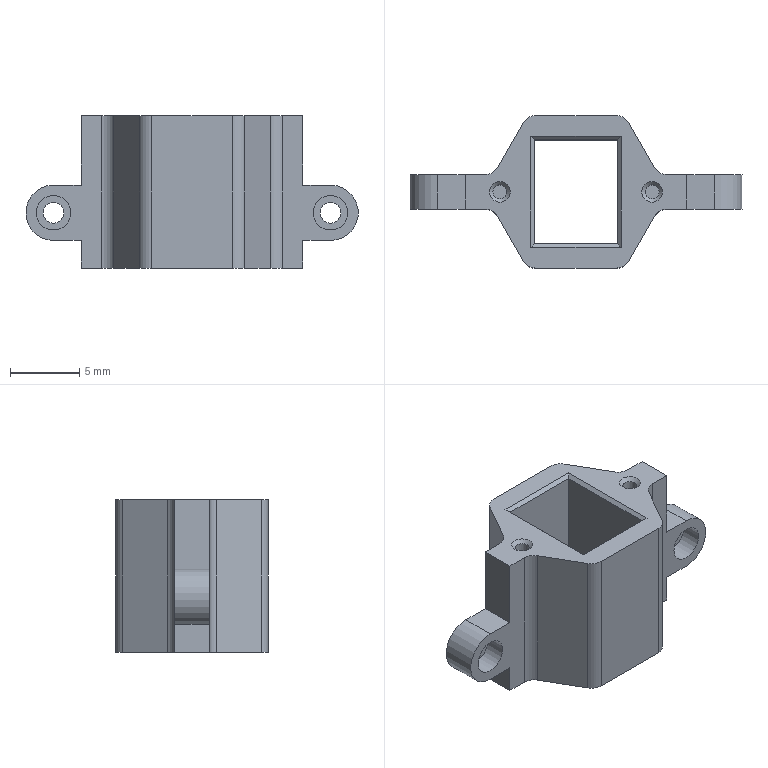Part | NX | features DATUM_CSYS 4, EXTRUDE 3, SKETCH 3, CBORE_HOLE 2, HOLE PACKAGE 2, BLEND 1, CHAMFER 1, SCALE 1 | 1 solid | 50 faces | box 24 x 11 x 11 mm | volume 869.205 mm3 | plane 32 | cylinder 16 | cone 2 | commonest cylinder face diameters 2 x8 1 x2 1.5 x2 2.5 x2 4 x2
STEP:
#1=CARTESIAN_POINT('',(-8.,-1.25,6.));
#2=VERTEX_POINT('',#1);
#3=CARTESIAN_POINT('',(-8.,1.25,6.));
#4=VERTEX_POINT('',#3);
#5=CARTESIAN_POINT('',(-8.,-1.25,6.));
#6=DIRECTION('',(0.,1.,0.));
#7=VECTOR('',#6,1000.);
#8=LINE('',#5,#7);
#9=EDGE_CURVE('',#2,#4,#8,.T.);
#10=ORIENTED_EDGE('',*,*,#9,.F.);
#11=CARTESIAN_POINT('',(-8.,-1.25,11.));
#12=VERTEX_POINT('',#11);
#13=CARTESIAN_POINT('',(-8.,-1.25,11.));
#14=DIRECTION('',(0.,0.,-1.));
#15=VECTOR('',#14,1000.);
#16=LINE('',#13,#15);
#17=EDGE_CURVE('',#12,#2,#16,.T.);
#18=ORIENTED_EDGE('',*,*,#17,.F.);
#19=CARTESIAN_POINT('',(-8.,1.25,11.));
#20=VERTEX_POINT('',#19);
#21=CARTESIAN_POINT('',(-8.,1.25,11.));
#22=DIRECTION('',(0.,-1.,0.));
#23=VECTOR('',#22,1000.);
#24=LINE('',#21,#23);
#25=EDGE_CURVE('',#20,#12,#24,.T.);
#26=ORIENTED_EDGE('',*,*,#25,.F.);
#27=CARTESIAN_POINT('',(-8.,1.25,11.));
#28=DIRECTION('',(0.,0.,-1.));
#29=VECTOR('',#28,1000.);
#30=LINE('',#27,#29);
#31=EDGE_CURVE('',#20,#4,#30,.T.);
#32=ORIENTED_EDGE('',*,*,#31,.T.);
#33=EDGE_LOOP('',(#10,#18,#26,#32));
#34=FACE_BOUND('',#33,.T.);
#35=CARTESIAN_POINT('',(-8.,1.25,11.));
#36=DIRECTION('',(1.,0.,0.));
#37=DIRECTION('',(0.,0.,-1.));
#38=AXIS2_PLACEMENT_3D('',#35,#36,#37);
#39=PLANE('',#38);
#40=ADVANCED_FACE('',(#34),#39,.F.);
#41=CARTESIAN_POINT('',(8.,-1.25,2.));
#42=VERTEX_POINT('',#41);
#43=CARTESIAN_POINT('',(8.,1.25,2.));
#44=VERTEX_POINT('',#43);
#45=CARTESIAN_POINT('',(8.,-1.25,2.));
#46=DIRECTION('',(0.,1.,0.));
#47=VECTOR('',#46,1000.);
#48=LINE('',#45,#47);
#49=EDGE_CURVE('',#42,#44,#48,.T.);
#50=ORIENTED_EDGE('',*,*,#49,.F.);
#51=CARTESIAN_POINT('',(8.,-1.25,0.));
#52=VERTEX_POINT('',#51);
#53=CARTESIAN_POINT('',(8.,-1.25,11.));
#54=DIRECTION('',(0.,0.,-1.));
#55=VECTOR('',#54,1000.);
#56=LINE('',#53,#55);
#57=EDGE_CURVE('',#42,#52,#56,.T.);
#58=ORIENTED_EDGE('',*,*,#57,.T.);
#59=CARTESIAN_POINT('',(8.,1.25,0.));
#60=VERTEX_POINT('',#59);
#61=CARTESIAN_POINT('',(8.,-1.25,0.));
#62=DIRECTION('',(0.,1.,0.));
#63=VECTOR('',#62,1000.);
#64=LINE('',#61,#63);
#65=EDGE_CURVE('',#52,#60,#64,.T.);
#66=ORIENTED_EDGE('',*,*,#65,.T.);
#67=CARTESIAN_POINT('',(8.,1.25,11.));
#68=DIRECTION('',(0.,0.,-1.));
#69=VECTOR('',#68,1000.);
#70=LINE('',#67,#69);
#71=EDGE_CURVE('',#44,#60,#70,.T.);
#72=ORIENTED_EDGE('',*,*,#71,.F.);
#73=EDGE_LOOP('',(#50,#58,#66,#72));
#74=FACE_BOUND('',#73,.T.);
#75=CARTESIAN_POINT('',(8.,-1.25,11.));
#76=DIRECTION('',(-1.,0.,0.));
#77=DIRECTION('',(0.,0.,1.));
#78=AXIS2_PLACEMENT_3D('',#75,#76,#77);
#79=PLANE('',#78);
#80=ADVANCED_FACE('',(#74),#79,.F.);
#81=CARTESIAN_POINT('',(-3.,3.75,10.75));
#82=VERTEX_POINT('',#81);
#83=CARTESIAN_POINT('',(-3.,3.75,0.));
#84=VERTEX_POINT('',#83);
#85=CARTESIAN_POINT('',(-3.,3.75,11.));
#86=DIRECTION('',(0.,0.,-1.));
#87=VECTOR('',#86,1000.);
#88=LINE('',#85,#87);
#89=EDGE_CURVE('',#82,#84,#88,.T.);
#90=ORIENTED_EDGE('',*,*,#89,.F.);
#91=CARTESIAN_POINT('',(-3.,-3.75,10.75));
#92=VERTEX_POINT('',#91);
#93=CARTESIAN_POINT('',(-3.,-3.75,10.75));
#94=DIRECTION('',(0.,-1.,0.));
#95=VECTOR('',#94,1000.);
#96=LINE('',#93,#95);
#97=EDGE_CURVE('',#82,#92,#96,.T.);
#98=ORIENTED_EDGE('',*,*,#97,.T.);
#99=CARTESIAN_POINT('',(-3.,-3.75,0.));
#100=VERTEX_POINT('',#99);
#101=CARTESIAN_POINT('',(-3.,-3.75,11.));
#102=DIRECTION('',(0.,0.,-1.));
#103=VECTOR('',#102,1000.);
#104=LINE('',#101,#103);
#105=EDGE_CURVE('',#92,#100,#104,.T.);
#106=ORIENTED_EDGE('',*,*,#105,.T.);
#107=CARTESIAN_POINT('',(-3.,-3.75,0.));
#108=DIRECTION('',(0.,1.,0.));
#109=VECTOR('',#108,1000.);
#110=LINE('',#107,#109);
#111=EDGE_CURVE('',#100,#84,#110,.T.);
#112=ORIENTED_EDGE('',*,*,#111,.T.);
#113=EDGE_LOOP('',(#90,#98,#106,#112));
#114=FACE_BOUND('',#113,.T.);
#115=CARTESIAN_POINT('',(-3.,-3.75,11.));
#116=DIRECTION('',(-1.,0.,0.));
#117=DIRECTION('',(0.,0.,1.));
#118=AXIS2_PLACEMENT_3D('',#115,#116,#117);
#119=PLANE('',#118);
#120=ADVANCED_FACE('',(#114),#119,.F.);
#121=CARTESIAN_POINT('',(3.,3.75,10.75));
#122=VERTEX_POINT('',#121);
#123=CARTESIAN_POINT('',(3.,3.75,0.));
#124=VERTEX_POINT('',#123);
#125=CARTESIAN_POINT('',(3.,3.75,11.));
#126=DIRECTION('',(0.,0.,-1.));
#127=VECTOR('',#126,1000.);
#128=LINE('',#125,#127);
#129=EDGE_CURVE('',#122,#124,#128,.T.);
#130=ORIENTED_EDGE('',*,*,#129,.F.);
#131=CARTESIAN_POINT('',(-3.,3.75,10.75));
#132=DIRECTION('',(-1.,0.,0.));
#133=VECTOR('',#132,1000.);
#134=LINE('',#131,#133);
#135=EDGE_CURVE('',#122,#82,#134,.T.);
#136=ORIENTED_EDGE('',*,*,#135,.T.);
#137=ORIENTED_EDGE('',*,*,#89,.T.);
#138=CARTESIAN_POINT('',(-3.,3.75,0.));
#139=DIRECTION('',(1.,0.,0.));
#140=VECTOR('',#139,1000.);
#141=LINE('',#138,#140);
#142=EDGE_CURVE('',#84,#124,#141,.T.);
#143=ORIENTED_EDGE('',*,*,#142,.T.);
#144=EDGE_LOOP('',(#130,#136,#137,#143));
#145=FACE_BOUND('',#144,.T.);
#146=CARTESIAN_POINT('',(-3.,3.75,11.));
#147=DIRECTION('',(0.,1.,0.));
#148=DIRECTION('',(0.,0.,1.));
#149=AXIS2_PLACEMENT_3D('',#146,#147,#148);
#150=PLANE('',#149);
#151=ADVANCED_FACE('',(#145),#150,.F.);
#152=CARTESIAN_POINT('',(3.,-3.75,10.75));
#153=VERTEX_POINT('',#152);
#154=CARTESIAN_POINT('',(3.,-3.75,0.));
#155=VERTEX_POINT('',#154);
#156=CARTESIAN_POINT('',(3.,-3.75,11.));
#157=DIRECTION('',(0.,0.,-1.));
#158=VECTOR('',#157,1000.);
#159=LINE('',#156,#158);
#160=EDGE_CURVE('',#153,#155,#159,.T.);
#161=ORIENTED_EDGE('',*,*,#160,.F.);
#162=CARTESIAN_POINT('',(3.,3.75,10.75));
#163=DIRECTION('',(0.,1.,0.));
#164=VECTOR('',#163,1000.);
#165=LINE('',#162,#164);
#166=EDGE_CURVE('',#153,#122,#165,.T.);
#167=ORIENTED_EDGE('',*,*,#166,.T.);
#168=ORIENTED_EDGE('',*,*,#129,.T.);
#169=CARTESIAN_POINT('',(3.,3.75,0.));
#170=DIRECTION('',(0.,-1.,0.));
#171=VECTOR('',#170,1000.);
#172=LINE('',#169,#171);
#173=EDGE_CURVE('',#124,#155,#172,.T.);
#174=ORIENTED_EDGE('',*,*,#173,.T.);
#175=EDGE_LOOP('',(#161,#167,#168,#174));
#176=FACE_BOUND('',#175,.T.);
#177=CARTESIAN_POINT('',(3.,3.75,11.));
#178=DIRECTION('',(1.,0.,0.));
#179=DIRECTION('',(0.,0.,-1.));
#180=AXIS2_PLACEMENT_3D('',#177,#178,#179);
#181=PLANE('',#180);
#182=ADVANCED_FACE('',(#176),#181,.F.);
#183=CARTESIAN_POINT('',(-8.,-1.25,2.));
#184=VERTEX_POINT('',#183);
#185=CARTESIAN_POINT('',(-8.,-1.25,0.));
#186=VERTEX_POINT('',#185);
#187=CARTESIAN_POINT('',(-8.,-1.25,11.));
#188=DIRECTION('',(0.,0.,-1.));
#189=VECTOR('',#188,1000.);
#190=LINE('',#187,#189);
#191=EDGE_CURVE('',#184,#186,#190,.T.);
#192=ORIENTED_EDGE('',*,*,#191,.F.);
#193=CARTESIAN_POINT('',(-8.,1.25,2.));
#194=VERTEX_POINT('',#193);
#195=CARTESIAN_POINT('',(-8.,-1.25,2.));
#196=DIRECTION('',(0.,1.,0.));
#197=VECTOR('',#196,1000.);
#198=LINE('',#195,#197);
#199=EDGE_CURVE('',#184,#194,#198,.T.);
#200=ORIENTED_EDGE('',*,*,#199,.T.);
#201=CARTESIAN_POINT('',(-8.,1.25,0.));
#202=VERTEX_POINT('',#201);
#203=CARTESIAN_POINT('',(-8.,1.25,11.));
#204=DIRECTION('',(0.,0.,-1.));
#205=VECTOR('',#204,1000.);
#206=LINE('',#203,#205);
#207=EDGE_CURVE('',#194,#202,#206,.T.);
#208=ORIENTED_EDGE('',*,*,#207,.T.);
#209=CARTESIAN_POINT('',(-8.,1.25,0.));
#210=DIRECTION('',(0.,-1.,0.));
#211=VECTOR('',#210,1000.);
#212=LINE('',#209,#211);
#213=EDGE_CURVE('',#202,#186,#212,.T.);
#214=ORIENTED_EDGE('',*,*,#213,.T.);
#215=EDGE_LOOP('',(#192,#200,#208,#214));
#216=FACE_BOUND('',#215,.T.);
#217=CARTESIAN_POINT('',(-8.,1.25,11.));
#218=DIRECTION('',(1.,0.,0.));
#219=DIRECTION('',(0.,0.,-1.));
#220=AXIS2_PLACEMENT_3D('',#217,#218,#219);
#221=PLANE('',#220);
#222=ADVANCED_FACE('',(#216),#221,.F.);
#223=CARTESIAN_POINT('',(-11.25,-1.25,4.));
#224=VERTEX_POINT('',#223);
#225=CARTESIAN_POINT('',(-10.,-1.25,4.));
#226=DIRECTION('',(0.,1.,0.));
#227=DIRECTION('',(-1.,0.,0.));
#228=AXIS2_PLACEMENT_3D('',#225,#226,#227);
#229=CIRCLE('',#228,1.25);
#230=EDGE_CURVE('',#224,#224,#229,.T.);
#231=ORIENTED_EDGE('',*,*,#230,.T.);
#232=EDGE_LOOP('',(#231));
#233=FACE_BOUND('',#232,.T.);
#234=CARTESIAN_POINT('',(-6.531,-1.25,0.));
#235=VERTEX_POINT('',#234);
#236=CARTESIAN_POINT('',(-8.,-1.25,0.));
#237=DIRECTION('',(1.,0.,0.));
#238=VECTOR('',#237,1000.);
#239=LINE('',#236,#238);
#240=EDGE_CURVE('',#186,#235,#239,.T.);
#241=ORIENTED_EDGE('',*,*,#240,.T.);
#242=CARTESIAN_POINT('',(-6.531,-1.25,11.));
#243=VERTEX_POINT('',#242);
#244=CARTESIAN_POINT('',(-6.531,-1.25,11.));
#245=DIRECTION('',(0.,0.,-1.));
#246=VECTOR('',#245,1000.);
#247=LINE('',#244,#246);
#248=EDGE_CURVE('',#235,#243,#247,.F.);
#249=ORIENTED_EDGE('',*,*,#248,.T.);
#250=CARTESIAN_POINT('',(-8.,-1.25,11.));
#251=DIRECTION('',(1.,0.,0.));
#252=VECTOR('',#251,1000.);
#253=LINE('',#250,#252);
#254=EDGE_CURVE('',#12,#243,#253,.T.);
#255=ORIENTED_EDGE('',*,*,#254,.F.);
#256=ORIENTED_EDGE('',*,*,#17,.T.);
#257=CARTESIAN_POINT('',(-10.,-1.25,6.));
#258=VERTEX_POINT('',#257);
#259=CARTESIAN_POINT('',(-8.,-1.25,6.));
#260=DIRECTION('',(-1.,0.,0.));
#261=VECTOR('',#260,1000.);
#262=LINE('',#259,#261);
#263=EDGE_CURVE('',#2,#258,#262,.T.);
#264=ORIENTED_EDGE('',*,*,#263,.T.);
#265=CARTESIAN_POINT('',(-10.,-1.25,2.));
#266=VERTEX_POINT('',#265);
#267=CARTESIAN_POINT('',(-10.,-1.25,4.));
#268=DIRECTION('',(0.,-1.,0.));
#269=DIRECTION('',(-1.,0.,0.));
#270=AXIS2_PLACEMENT_3D('',#267,#268,#269);
#271=CIRCLE('',#270,2.);
#272=EDGE_CURVE('',#258,#266,#271,.T.);
#273=ORIENTED_EDGE('',*,*,#272,.T.);
#274=CARTESIAN_POINT('',(-10.,-1.25,2.));
#275=DIRECTION('',(1.,0.,0.));
#276=VECTOR('',#275,1000.);
#277=LINE('',#274,#276);
#278=EDGE_CURVE('',#266,#184,#277,.T.);
#279=ORIENTED_EDGE('',*,*,#278,.T.);
#280=ORIENTED_EDGE('',*,*,#191,.T.);
#281=EDGE_LOOP('',(#241,#249,#255,#256,#264,#273,#279,#280));
#282=FACE_BOUND('',#281,.T.);
#283=CARTESIAN_POINT('',(-8.,-1.25,11.));
#284=DIRECTION('',(0.,1.,0.));
#285=DIRECTION('',(-1.,0.,0.));
#286=AXIS2_PLACEMENT_3D('',#283,#284,#285);
#287=PLANE('',#286);
#288=ADVANCED_FACE('',(#233,#282),#287,.F.);
#289=CARTESIAN_POINT('',(-5.665,-1.75,11.));
#290=VERTEX_POINT('',#289);
#291=CARTESIAN_POINT('',(-3.789,-5.,11.));
#292=VERTEX_POINT('',#291);
#293=CARTESIAN_POINT('',(-5.954,-1.25,11.));
#294=DIRECTION('',(0.5,-0.866,0.));
#295=VECTOR('',#294,1000.);
#296=LINE('',#293,#295);
#297=EDGE_CURVE('',#290,#292,#296,.T.);
#298=ORIENTED_EDGE('',*,*,#297,.F.);
#299=CARTESIAN_POINT('',(-5.665,-1.75,0.));
#300=VERTEX_POINT('',#299);
#301=CARTESIAN_POINT('',(-5.665,-1.75,0.));
#302=DIRECTION('',(0.,0.,-1.));
#303=VECTOR('',#302,1000.);
#304=LINE('',#301,#303);
#305=EDGE_CURVE('',#290,#300,#304,.T.);
#306=ORIENTED_EDGE('',*,*,#305,.T.);
#307=CARTESIAN_POINT('',(-3.789,-5.,0.));
#308=VERTEX_POINT('',#307);
#309=CARTESIAN_POINT('',(-5.954,-1.25,0.));
#310=DIRECTION('',(0.5,-0.866,0.));
#311=VECTOR('',#310,1000.);
#312=LINE('',#309,#311);
#313=EDGE_CURVE('',#300,#308,#312,.T.);
#314=ORIENTED_EDGE('',*,*,#313,.T.);
#315=CARTESIAN_POINT('',(-3.789,-5.,11.));
#316=DIRECTION('',(0.,0.,-1.));
#317=VECTOR('',#316,1000.);
#318=LINE('',#315,#317);
#319=EDGE_CURVE('',#308,#292,#318,.F.);
#320=ORIENTED_EDGE('',*,*,#319,.T.);
#321=EDGE_LOOP('',(#298,#306,#314,#320));
#322=FACE_BOUND('',#321,.T.);
#323=CARTESIAN_POINT('',(-5.954,-1.25,11.));
#324=DIRECTION('',(0.866,0.5,0.));
#325=DIRECTION('',(-0.5,0.866,0.));
#326=AXIS2_PLACEMENT_3D('',#323,#324,#325);
#327=PLANE('',#326);
#328=ADVANCED_FACE('',(#322),#327,.F.);
#329=CARTESIAN_POINT('',(-2.923,-5.5,0.));
#330=VERTEX_POINT('',#329);
#331=CARTESIAN_POINT('',(2.923,-5.5,0.));
#332=VERTEX_POINT('',#331);
#333=CARTESIAN_POINT('',(-3.5,-5.5,0.));
#334=DIRECTION('',(1.,0.,0.));
#335=VECTOR('',#334,1000.);
#336=LINE('',#333,#335);
#337=EDGE_CURVE('',#330,#332,#336,.T.);
#338=ORIENTED_EDGE('',*,*,#337,.T.);
#339=CARTESIAN_POINT('',(2.923,-5.5,11.));
#340=VERTEX_POINT('',#339);
#341=CARTESIAN_POINT('',(2.923,-5.5,11.));
#342=DIRECTION('',(0.,0.,-1.));
#343=VECTOR('',#342,1000.);
#344=LINE('',#341,#343);
#345=EDGE_CURVE('',#332,#340,#344,.F.);
#346=ORIENTED_EDGE('',*,*,#345,.T.);
#347=CARTESIAN_POINT('',(-2.923,-5.5,11.));
#348=VERTEX_POINT('',#347);
#349=CARTESIAN_POINT('',(-3.5,-5.5,11.));
#350=DIRECTION('',(1.,0.,0.));
#351=VECTOR('',#350,1000.);
#352=LINE('',#349,#351);
#353=EDGE_CURVE('',#348,#340,#352,.T.);
#354=ORIENTED_EDGE('',*,*,#353,.F.);
#355=CARTESIAN_POINT('',(-2.923,-5.5,11.));
#356=DIRECTION('',(0.,0.,-1.));
#357=VECTOR('',#356,1000.);
#358=LINE('',#355,#357);
#359=EDGE_CURVE('',#348,#330,#358,.T.);
#360=ORIENTED_EDGE('',*,*,#359,.T.);
#361=EDGE_LOOP('',(#338,#346,#354,#360));
#362=FACE_BOUND('',#361,.T.);
#363=CARTESIAN_POINT('',(-3.5,-5.5,11.));
#364=DIRECTION('',(0.,1.,0.));
#365=DIRECTION('',(0.,0.,1.));
#366=AXIS2_PLACEMENT_3D('',#363,#364,#365);
#367=PLANE('',#366);
#368=ADVANCED_FACE('',(#362),#367,.F.);
#369=CARTESIAN_POINT('',(3.789,-5.,0.));
#370=VERTEX_POINT('',#369);
#371=CARTESIAN_POINT('',(5.665,-1.75,0.));
#372=VERTEX_POINT('',#371);
#373=CARTESIAN_POINT('',(3.5,-5.5,0.));
#374=DIRECTION('',(0.5,0.866,0.));
#375=VECTOR('',#374,1000.);
#376=LINE('',#373,#375);
#377=EDGE_CURVE('',#370,#372,#376,.T.);
#378=ORIENTED_EDGE('',*,*,#377,.T.);
#379=CARTESIAN_POINT('',(5.665,-1.75,11.));
#380=VERTEX_POINT('',#379);
#381=CARTESIAN_POINT('',(5.665,-1.75,11.));
#382=DIRECTION('',(0.,0.,-1.));
#383=VECTOR('',#382,1000.);
#384=LINE('',#381,#383);
#385=EDGE_CURVE('',#372,#380,#384,.F.);
#386=ORIENTED_EDGE('',*,*,#385,.T.);
#387=CARTESIAN_POINT('',(3.789,-5.,11.));
#388=VERTEX_POINT('',#387);
#389=CARTESIAN_POINT('',(3.5,-5.5,11.));
#390=DIRECTION('',(0.5,0.866,0.));
#391=VECTOR('',#390,1000.);
#392=LINE('',#389,#391);
#393=EDGE_CURVE('',#388,#380,#392,.T.);
#394=ORIENTED_EDGE('',*,*,#393,.F.);
#395=CARTESIAN_POINT('',(3.789,-5.,11.));
#396=DIRECTION('',(0.,0.,-1.));
#397=VECTOR('',#396,1000.);
#398=LINE('',#395,#397);
#399=EDGE_CURVE('',#388,#370,#398,.T.);
#400=ORIENTED_EDGE('',*,*,#399,.T.);
#401=EDGE_LOOP('',(#378,#386,#394,#400));
#402=FACE_BOUND('',#401,.T.);
#403=CARTESIAN_POINT('',(3.5,-5.5,11.));
#404=DIRECTION('',(-0.866,0.5,0.));
#405=DIRECTION('',(-0.5,-0.866,0.));
#406=AXIS2_PLACEMENT_3D('',#403,#404,#405);
#407=PLANE('',#406);
#408=ADVANCED_FACE('',(#402),#407,.F.);
#409=CARTESIAN_POINT('',(8.75,-1.25,4.));
#410=VERTEX_POINT('',#409);
#411=CARTESIAN_POINT('',(10.,-1.25,4.));
#412=DIRECTION('',(0.,1.,0.));
#413=DIRECTION('',(-1.,0.,0.));
#414=AXIS2_PLACEMENT_3D('',#411,#412,#413);
#415=CIRCLE('',#414,1.25);
#416=EDGE_CURVE('',#410,#410,#415,.T.);
#417=ORIENTED_EDGE('',*,*,#416,.T.);
#418=EDGE_LOOP('',(#417));
#419=FACE_BOUND('',#418,.T.);
#420=CARTESIAN_POINT('',(6.531,-1.25,11.));
#421=VERTEX_POINT('',#420);
#422=CARTESIAN_POINT('',(8.,-1.25,11.));
#423=VERTEX_POINT('',#422);
#424=CARTESIAN_POINT('',(5.954,-1.25,11.));
#425=DIRECTION('',(1.,0.,0.));
#426=VECTOR('',#425,1000.);
#427=LINE('',#424,#426);
#428=EDGE_CURVE('',#421,#423,#427,.T.);
#429=ORIENTED_EDGE('',*,*,#428,.F.);
#430=CARTESIAN_POINT('',(6.531,-1.25,0.));
#431=VERTEX_POINT('',#430);
#432=CARTESIAN_POINT('',(6.531,-1.25,0.));
#433=DIRECTION('',(0.,0.,-1.));
#434=VECTOR('',#433,1000.);
#435=LINE('',#432,#434);
#436=EDGE_CURVE('',#421,#431,#435,.T.);
#437=ORIENTED_EDGE('',*,*,#436,.T.);
#438=CARTESIAN_POINT('',(5.954,-1.25,0.));
#439=DIRECTION('',(1.,0.,0.));
#440=VECTOR('',#439,1000.);
#441=LINE('',#438,#440);
#442=EDGE_CURVE('',#431,#52,#441,.T.);
#443=ORIENTED_EDGE('',*,*,#442,.T.);
#444=ORIENTED_EDGE('',*,*,#57,.F.);
#445=CARTESIAN_POINT('',(10.,-1.25,2.));
#446=VERTEX_POINT('',#445);
#447=CARTESIAN_POINT('',(10.,-1.25,2.));
#448=DIRECTION('',(-1.,0.,0.));
#449=VECTOR('',#448,1000.);
#450=LINE('',#447,#449);
#451=EDGE_CURVE('',#446,#42,#450,.T.);
#452=ORIENTED_EDGE('',*,*,#451,.F.);
#453=CARTESIAN_POINT('',(10.,-1.25,6.));
#454=VERTEX_POINT('',#453);
#455=CARTESIAN_POINT('',(10.,-1.25,4.));
#456=DIRECTION('',(0.,1.,0.));
#457=DIRECTION('',(1.,0.,0.));
#458=AXIS2_PLACEMENT_3D('',#455,#456,#457);
#459=CIRCLE('',#458,2.);
#460=EDGE_CURVE('',#454,#446,#459,.T.);
#461=ORIENTED_EDGE('',*,*,#460,.F.);
#462=CARTESIAN_POINT('',(8.,-1.25,6.));
#463=VERTEX_POINT('',#462);
#464=CARTESIAN_POINT('',(8.,-1.25,6.));
#465=DIRECTION('',(1.,0.,0.));
#466=VECTOR('',#465,1000.);
#467=LINE('',#464,#466);
#468=EDGE_CURVE('',#463,#454,#467,.T.);
#469=ORIENTED_EDGE('',*,*,#468,.F.);
#470=CARTESIAN_POINT('',(8.,-1.25,11.));
#471=DIRECTION('',(0.,0.,-1.));
#472=VECTOR('',#471,1000.);
#473=LINE('',#470,#472);
#474=EDGE_CURVE('',#423,#463,#473,.T.);
#475=ORIENTED_EDGE('',*,*,#474,.F.);
#476=EDGE_LOOP('',(#429,#437,#443,#444,#452,#461,#469,#475));
#477=FACE_BOUND('',#476,.T.);
#478=CARTESIAN_POINT('',(5.954,-1.25,11.));
#479=DIRECTION('',(0.,1.,0.));
#480=DIRECTION('',(-1.,0.,0.));
#481=AXIS2_PLACEMENT_3D('',#478,#479,#480);
#482=PLANE('',#481);
#483=ADVANCED_FACE('',(#419,#477),#482,.F.);
#484=ORIENTED_EDGE('',*,*,#474,.T.);
#485=CARTESIAN_POINT('',(8.,1.25,6.));
#486=VERTEX_POINT('',#485);
#487=CARTESIAN_POINT('',(8.,-1.25,6.));
#488=DIRECTION('',(0.,1.,0.));
#489=VECTOR('',#488,1000.);
#490=LINE('',#487,#489);
#491=EDGE_CURVE('',#463,#486,#490,.T.);
#492=ORIENTED_EDGE('',*,*,#491,.T.);
#493=CARTESIAN_POINT('',(8.,1.25,11.));
#494=VERTEX_POINT('',#493);
#495=CARTESIAN_POINT('',(8.,1.25,11.));
#496=DIRECTION('',(0.,0.,-1.));
#497=VECTOR('',#496,1000.);
#498=LINE('',#495,#497);
#499=EDGE_CURVE('',#494,#486,#498,.T.);
#500=ORIENTED_EDGE('',*,*,#499,.F.);
#501=CARTESIAN_POINT('',(8.,-1.25,11.));
#502=DIRECTION('',(0.,1.,0.));
#503=VECTOR('',#502,1000.);
#504=LINE('',#501,#503);
#505=EDGE_CURVE('',#423,#494,#504,.T.);
#506=ORIENTED_EDGE('',*,*,#505,.F.);
#507=EDGE_LOOP('',(#484,#492,#500,#506));
#508=FACE_BOUND('',#507,.T.);
#509=CARTESIAN_POINT('',(8.,-1.25,11.));
#510=DIRECTION('',(-1.,0.,0.));
#511=DIRECTION('',(0.,0.,1.));
#512=AXIS2_PLACEMENT_3D('',#509,#510,#511);
#513=PLANE('',#512);
#514=ADVANCED_FACE('',(#508),#513,.F.);
#515=CARTESIAN_POINT('',(10.75,1.25,4.));
#516=VERTEX_POINT('',#515);
#517=CARTESIAN_POINT('',(10.,1.25,4.));
#518=DIRECTION('',(0.,-1.,0.));
#519=DIRECTION('',(1.,0.,0.));
#520=AXIS2_PLACEMENT_3D('',#517,#518,#519);
#521=CIRCLE('',#520,0.75);
#522=EDGE_CURVE('',#516,#516,#521,.T.);
#523=ORIENTED_EDGE('',*,*,#522,.T.);
#524=EDGE_LOOP('',(#523));
#525=FACE_BOUND('',#524,.T.);
#526=CARTESIAN_POINT('',(6.531,1.25,0.));
#527=VERTEX_POINT('',#526);
#528=CARTESIAN_POINT('',(8.,1.25,0.));
#529=DIRECTION('',(-1.,0.,0.));
#530=VECTOR('',#529,1000.);
#531=LINE('',#528,#530);
#532=EDGE_CURVE('',#60,#527,#531,.T.);
#533=ORIENTED_EDGE('',*,*,#532,.T.);
#534=CARTESIAN_POINT('',(6.531,1.25,11.));
#535=VERTEX_POINT('',#534);
#536=CARTESIAN_POINT('',(6.531,1.25,11.));
#537=DIRECTION('',(0.,0.,-1.));
#538=VECTOR('',#537,1000.);
#539=LINE('',#536,#538);
#540=EDGE_CURVE('',#527,#535,#539,.F.);
#541=ORIENTED_EDGE('',*,*,#540,.T.);
#542=CARTESIAN_POINT('',(8.,1.25,11.));
#543=DIRECTION('',(-1.,0.,0.));
#544=VECTOR('',#543,1000.);
#545=LINE('',#542,#544);
#546=EDGE_CURVE('',#494,#535,#545,.T.);
#547=ORIENTED_EDGE('',*,*,#546,.F.);
#548=ORIENTED_EDGE('',*,*,#499,.T.);
#549=CARTESIAN_POINT('',(10.,1.25,6.));
#550=VERTEX_POINT('',#549);
#551=CARTESIAN_POINT('',(8.,1.25,6.));
#552=DIRECTION('',(1.,0.,0.));
#553=VECTOR('',#552,1000.);
#554=LINE('',#551,#553);
#555=EDGE_CURVE('',#486,#550,#554,.T.);
#556=ORIENTED_EDGE('',*,*,#555,.T.);
#557=CARTESIAN_POINT('',(10.,1.25,2.));
#558=VERTEX_POINT('',#557);
#559=CARTESIAN_POINT('',(10.,1.25,4.));
#560=DIRECTION('',(0.,1.,0.));
#561=DIRECTION('',(1.,0.,0.));
#562=AXIS2_PLACEMENT_3D('',#559,#560,#561);
#563=CIRCLE('',#562,2.);
#564=EDGE_CURVE('',#550,#558,#563,.T.);
#565=ORIENTED_EDGE('',*,*,#564,.T.);
#566=CARTESIAN_POINT('',(10.,1.25,2.));
#567=DIRECTION('',(-1.,0.,0.));
#568=VECTOR('',#567,1000.);
#569=LINE('',#566,#568);
#570=EDGE_CURVE('',#558,#44,#569,.T.);
#571=ORIENTED_EDGE('',*,*,#570,.T.);
#572=ORIENTED_EDGE('',*,*,#71,.T.);
#573=EDGE_LOOP('',(#533,#541,#547,#548,#556,#565,#571,#572));
#574=FACE_BOUND('',#573,.T.);
#575=CARTESIAN_POINT('',(8.,1.25,11.));
#576=DIRECTION('',(0.,-1.,0.));
#577=DIRECTION('',(1.,0.,0.));
#578=AXIS2_PLACEMENT_3D('',#575,#576,#577);
#579=PLANE('',#578);
#580=ADVANCED_FACE('',(#525,#574),#579,.F.);
#581=CARTESIAN_POINT('',(5.665,1.75,0.));
#582=VERTEX_POINT('',#581);
#583=CARTESIAN_POINT('',(3.789,5.,0.));
#584=VERTEX_POINT('',#583);
#585=CARTESIAN_POINT('',(5.954,1.25,0.));
#586=DIRECTION('',(-0.5,0.866,0.));
#587=VECTOR('',#586,1000.);
#588=LINE('',#585,#587);
#589=EDGE_CURVE('',#582,#584,#588,.T.);
#590=ORIENTED_EDGE('',*,*,#589,.T.);
#591=CARTESIAN_POINT('',(3.789,5.,11.));
#592=VERTEX_POINT('',#591);
#593=CARTESIAN_POINT('',(3.789,5.,11.));
#594=DIRECTION('',(0.,0.,-1.));
#595=VECTOR('',#594,1000.);
#596=LINE('',#593,#595);
#597=EDGE_CURVE('',#584,#592,#596,.F.);
#598=ORIENTED_EDGE('',*,*,#597,.T.);
#599=CARTESIAN_POINT('',(5.665,1.75,11.));
#600=VERTEX_POINT('',#599);
#601=CARTESIAN_POINT('',(5.954,1.25,11.));
#602=DIRECTION('',(-0.5,0.866,0.));
#603=VECTOR('',#602,1000.);
#604=LINE('',#601,#603);
#605=EDGE_CURVE('',#600,#592,#604,.T.);
#606=ORIENTED_EDGE('',*,*,#605,.F.);
#607=CARTESIAN_POINT('',(5.665,1.75,0.));
#608=DIRECTION('',(0.,0.,-1.));
#609=VECTOR('',#608,1000.);
#610=LINE('',#607,#609);
#611=EDGE_CURVE('',#600,#582,#610,.T.);
#612=ORIENTED_EDGE('',*,*,#611,.T.);
#613=EDGE_LOOP('',(#590,#598,#606,#612));
#614=FACE_BOUND('',#613,.T.);
#615=CARTESIAN_POINT('',(5.954,1.25,11.));
#616=DIRECTION('',(-0.866,-0.5,0.));
#617=DIRECTION('',(0.5,-0.866,0.));
#618=AXIS2_PLACEMENT_3D('',#615,#616,#617);
#619=PLANE('',#618);
#620=ADVANCED_FACE('',(#614),#619,.F.);
#621=CARTESIAN_POINT('',(2.923,5.5,0.));
#622=VERTEX_POINT('',#621);
#623=CARTESIAN_POINT('',(-2.923,5.5,0.));
#624=VERTEX_POINT('',#623);
#625=CARTESIAN_POINT('',(3.5,5.5,0.));
#626=DIRECTION('',(-1.,0.,0.));
#627=VECTOR('',#626,1000.);
#628=LINE('',#625,#627);
#629=EDGE_CURVE('',#622,#624,#628,.T.);
#630=ORIENTED_EDGE('',*,*,#629,.T.);
#631=CARTESIAN_POINT('',(-2.923,5.5,11.));
#632=VERTEX_POINT('',#631);
#633=CARTESIAN_POINT('',(-2.923,5.5,11.));
#634=DIRECTION('',(0.,0.,-1.));
#635=VECTOR('',#634,1000.);
#636=LINE('',#633,#635);
#637=EDGE_CURVE('',#624,#632,#636,.F.);
#638=ORIENTED_EDGE('',*,*,#637,.T.);
#639=CARTESIAN_POINT('',(2.923,5.5,11.));
#640=VERTEX_POINT('',#639);
#641=CARTESIAN_POINT('',(3.5,5.5,11.));
#642=DIRECTION('',(-1.,0.,0.));
#643=VECTOR('',#642,1000.);
#644=LINE('',#641,#643);
#645=EDGE_CURVE('',#640,#632,#644,.T.);
#646=ORIENTED_EDGE('',*,*,#645,.F.);
#647=CARTESIAN_POINT('',(2.923,5.5,11.));
#648=DIRECTION('',(0.,0.,-1.));
#649=VECTOR('',#648,1000.);
#650=LINE('',#647,#649);
#651=EDGE_CURVE('',#640,#622,#650,.T.);
#652=ORIENTED_EDGE('',*,*,#651,.T.);
#653=EDGE_LOOP('',(#630,#638,#646,#652));
#654=FACE_BOUND('',#653,.T.);
#655=CARTESIAN_POINT('',(3.5,5.5,11.));
#656=DIRECTION('',(0.,-1.,0.));
#657=DIRECTION('',(0.,0.,-1.));
#658=AXIS2_PLACEMENT_3D('',#655,#656,#657);
#659=PLANE('',#658);
#660=ADVANCED_FACE('',(#654),#659,.F.);
#661=CARTESIAN_POINT('',(-3.789,5.,0.));
#662=VERTEX_POINT('',#661);
#663=CARTESIAN_POINT('',(-5.665,1.75,0.));
#664=VERTEX_POINT('',#663);
#665=CARTESIAN_POINT('',(-3.5,5.5,0.));
#666=DIRECTION('',(-0.5,-0.866,0.));
#667=VECTOR('',#666,1000.);
#668=LINE('',#665,#667);
#669=EDGE_CURVE('',#662,#664,#668,.T.);
#670=ORIENTED_EDGE('',*,*,#669,.T.);
#671=CARTESIAN_POINT('',(-5.665,1.75,11.));
#672=VERTEX_POINT('',#671);
#673=CARTESIAN_POINT('',(-5.665,1.75,11.));
#674=DIRECTION('',(0.,0.,-1.));
#675=VECTOR('',#674,1000.);
#676=LINE('',#673,#675);
#677=EDGE_CURVE('',#664,#672,#676,.F.);
#678=ORIENTED_EDGE('',*,*,#677,.T.);
#679=CARTESIAN_POINT('',(-3.789,5.,11.));
#680=VERTEX_POINT('',#679);
#681=CARTESIAN_POINT('',(-3.5,5.5,11.));
#682=DIRECTION('',(-0.5,-0.866,0.));
#683=VECTOR('',#682,1000.);
#684=LINE('',#681,#683);
#685=EDGE_CURVE('',#680,#672,#684,.T.);
#686=ORIENTED_EDGE('',*,*,#685,.F.);
#687=CARTESIAN_POINT('',(-3.789,5.,11.));
#688=DIRECTION('',(0.,0.,-1.));
#689=VECTOR('',#688,1000.);
#690=LINE('',#687,#689);
#691=EDGE_CURVE('',#680,#662,#690,.T.);
#692=ORIENTED_EDGE('',*,*,#691,.T.);
#693=EDGE_LOOP('',(#670,#678,#686,#692));
#694=FACE_BOUND('',#693,.T.);
#695=CARTESIAN_POINT('',(-3.5,5.5,11.));
#696=DIRECTION('',(0.866,-0.5,0.));
#697=DIRECTION('',(0.5,0.866,0.));
#698=AXIS2_PLACEMENT_3D('',#695,#696,#697);
#699=PLANE('',#698);
#700=ADVANCED_FACE('',(#694),#699,.F.);
#701=CARTESIAN_POINT('',(-9.25,1.25,4.));
#702=VERTEX_POINT('',#701);
#703=CARTESIAN_POINT('',(-10.,1.25,4.));
#704=DIRECTION('',(0.,-1.,0.));
#705=DIRECTION('',(1.,0.,0.));
#706=AXIS2_PLACEMENT_3D('',#703,#704,#705);
#707=CIRCLE('',#706,0.75);
#708=EDGE_CURVE('',#702,#702,#707,.T.);
#709=ORIENTED_EDGE('',*,*,#708,.T.);
#710=EDGE_LOOP('',(#709));
#711=FACE_BOUND('',#710,.T.);
#712=CARTESIAN_POINT('',(-6.531,1.25,11.));
#713=VERTEX_POINT('',#712);
#714=CARTESIAN_POINT('',(-5.954,1.25,11.));
#715=DIRECTION('',(-1.,0.,0.));
#716=VECTOR('',#715,1000.);
#717=LINE('',#714,#716);
#718=EDGE_CURVE('',#713,#20,#717,.T.);
#719=ORIENTED_EDGE('',*,*,#718,.F.);
#720=CARTESIAN_POINT('',(-6.531,1.25,0.));
#721=VERTEX_POINT('',#720);
#722=CARTESIAN_POINT('',(-6.531,1.25,0.));
#723=DIRECTION('',(0.,0.,-1.));
#724=VECTOR('',#723,1000.);
#725=LINE('',#722,#724);
#726=EDGE_CURVE('',#713,#721,#725,.T.);
#727=ORIENTED_EDGE('',*,*,#726,.T.);
#728=CARTESIAN_POINT('',(-5.954,1.25,0.));
#729=DIRECTION('',(-1.,0.,0.));
#730=VECTOR('',#729,1000.);
#731=LINE('',#728,#730);
#732=EDGE_CURVE('',#721,#202,#731,.T.);
#733=ORIENTED_EDGE('',*,*,#732,.T.);
#734=ORIENTED_EDGE('',*,*,#207,.F.);
#735=CARTESIAN_POINT('',(-10.,1.25,2.));
#736=VERTEX_POINT('',#735);
#737=CARTESIAN_POINT('',(-10.,1.25,2.));
#738=DIRECTION('',(1.,0.,0.));
#739=VECTOR('',#738,1000.);
#740=LINE('',#737,#739);
#741=EDGE_CURVE('',#736,#194,#740,.T.);
#742=ORIENTED_EDGE('',*,*,#741,.F.);
#743=CARTESIAN_POINT('',(-10.,1.25,6.));
#744=VERTEX_POINT('',#743);
#745=CARTESIAN_POINT('',(-10.,1.25,4.));
#746=DIRECTION('',(0.,-1.,0.));
#747=DIRECTION('',(-1.,0.,0.));
#748=AXIS2_PLACEMENT_3D('',#745,#746,#747);
#749=CIRCLE('',#748,2.);
#750=EDGE_CURVE('',#744,#736,#749,.T.);
#751=ORIENTED_EDGE('',*,*,#750,.F.);
#752=CARTESIAN_POINT('',(-8.,1.25,6.));
#753=DIRECTION('',(-1.,0.,0.));
#754=VECTOR('',#753,1000.);
#755=LINE('',#752,#754);
#756=EDGE_CURVE('',#4,#744,#755,.T.);
#757=ORIENTED_EDGE('',*,*,#756,.F.);
#758=ORIENTED_EDGE('',*,*,#31,.F.);
#759=EDGE_LOOP('',(#719,#727,#733,#734,#742,#751,#757,#758));
#760=FACE_BOUND('',#759,.T.);
#761=CARTESIAN_POINT('',(-5.954,1.25,11.));
#762=DIRECTION('',(0.,-1.,0.));
#763=DIRECTION('',(1.,0.,0.));
#764=AXIS2_PLACEMENT_3D('',#761,#762,#763);
#765=PLANE('',#764);
#766=ADVANCED_FACE('',(#711,#760),#765,.F.);
#767=ORIENTED_EDGE('',*,*,#105,.F.);
#768=CARTESIAN_POINT('',(3.,-3.75,10.75));
#769=DIRECTION('',(1.,0.,0.));
#770=VECTOR('',#769,1000.);
#771=LINE('',#768,#770);
#772=EDGE_CURVE('',#92,#153,#771,.T.);
#773=ORIENTED_EDGE('',*,*,#772,.T.);
#774=ORIENTED_EDGE('',*,*,#160,.T.);
#775=CARTESIAN_POINT('',(3.,-3.75,0.));
#776=DIRECTION('',(-1.,0.,0.));
#777=VECTOR('',#776,1000.);
#778=LINE('',#775,#777);
#779=EDGE_CURVE('',#155,#100,#778,.T.);
#780=ORIENTED_EDGE('',*,*,#779,.T.);
#781=EDGE_LOOP('',(#767,#773,#774,#780));
#782=FACE_BOUND('',#781,.T.);
#783=CARTESIAN_POINT('',(3.,-3.75,11.));
#784=DIRECTION('',(0.,-1.,0.));
#785=DIRECTION('',(0.,0.,-1.));
#786=AXIS2_PLACEMENT_3D('',#783,#784,#785);
#787=PLANE('',#786);
#788=ADVANCED_FACE('',(#782),#787,.F.);
#789=CARTESIAN_POINT('',(-4.75,0.,11.));
#790=VERTEX_POINT('',#789);
#791=CARTESIAN_POINT('',(-5.5,0.,11.));
#792=DIRECTION('',(0.,0.,1.));
#793=DIRECTION('',(1.,0.,0.));
#794=AXIS2_PLACEMENT_3D('',#791,#792,#793);
#795=CIRCLE('',#794,0.75);
#796=EDGE_CURVE('',#790,#790,#795,.F.);
#797=ORIENTED_EDGE('',*,*,#796,.T.);
#798=EDGE_LOOP('',(#797));
#799=FACE_BOUND('',#798,.T.);
#800=CARTESIAN_POINT('',(6.25,0.,11.));
#801=VERTEX_POINT('',#800);
#802=CARTESIAN_POINT('',(5.5,0.,11.));
#803=DIRECTION('',(0.,0.,1.));
#804=DIRECTION('',(1.,0.,0.));
#805=AXIS2_PLACEMENT_3D('',#802,#803,#804);
#806=CIRCLE('',#805,0.75);
#807=EDGE_CURVE('',#801,#801,#806,.F.);
#808=ORIENTED_EDGE('',*,*,#807,.T.);
#809=EDGE_LOOP('',(#808));
#810=FACE_BOUND('',#809,.T.);
#811=CARTESIAN_POINT('',(-3.25,4.,11.));
#812=VERTEX_POINT('',#811);
#813=CARTESIAN_POINT('',(3.25,4.,11.));
#814=VERTEX_POINT('',#813);
#815=CARTESIAN_POINT('',(3.,4.,11.));
#816=DIRECTION('',(1.,0.,0.));
#817=VECTOR('',#816,1000.);
#818=LINE('',#815,#817);
#819=EDGE_CURVE('',#812,#814,#818,.T.);
#820=ORIENTED_EDGE('',*,*,#819,.T.);
#821=CARTESIAN_POINT('',(3.25,-4.,11.));
#822=VERTEX_POINT('',#821);
#823=CARTESIAN_POINT('',(3.25,-3.75,11.));
#824=DIRECTION('',(0.,-1.,0.));
#825=VECTOR('',#824,1000.);
#826=LINE('',#823,#825);
#827=EDGE_CURVE('',#814,#822,#826,.T.);
#828=ORIENTED_EDGE('',*,*,#827,.T.);
#829=CARTESIAN_POINT('',(-3.25,-4.,11.));
#830=VERTEX_POINT('',#829);
#831=CARTESIAN_POINT('',(-3.,-4.,11.));
#832=DIRECTION('',(-1.,0.,0.));
#833=VECTOR('',#832,1000.);
#834=LINE('',#831,#833);
#835=EDGE_CURVE('',#822,#830,#834,.T.);
#836=ORIENTED_EDGE('',*,*,#835,.T.);
#837=CARTESIAN_POINT('',(-3.25,3.75,11.));
#838=DIRECTION('',(0.,1.,0.));
#839=VECTOR('',#838,1000.);
#840=LINE('',#837,#839);
#841=EDGE_CURVE('',#830,#812,#840,.T.);
#842=ORIENTED_EDGE('',*,*,#841,.T.);
#843=EDGE_LOOP('',(#820,#828,#836,#842));
#844=FACE_BOUND('',#843,.T.);
#845=ORIENTED_EDGE('',*,*,#645,.T.);
#846=CARTESIAN_POINT('',(-2.923,4.5,11.));
#847=DIRECTION('',(0.,0.,1.));
#848=DIRECTION('',(1.,0.,0.));
#849=AXIS2_PLACEMENT_3D('',#846,#847,#848);
#850=CIRCLE('',#849,1.);
#851=EDGE_CURVE('',#632,#680,#850,.T.);
#852=ORIENTED_EDGE('',*,*,#851,.T.);
#853=ORIENTED_EDGE('',*,*,#685,.T.);
#854=CARTESIAN_POINT('',(-6.531,2.25,11.));
#855=DIRECTION('',(0.,0.,1.));
#856=DIRECTION('',(1.,0.,0.));
#857=AXIS2_PLACEMENT_3D('',#854,#855,#856);
#858=CIRCLE('',#857,1.);
#859=EDGE_CURVE('',#672,#713,#858,.F.);
#860=ORIENTED_EDGE('',*,*,#859,.T.);
#861=ORIENTED_EDGE('',*,*,#718,.T.);
#862=ORIENTED_EDGE('',*,*,#25,.T.);
#863=ORIENTED_EDGE('',*,*,#254,.T.);
#864=CARTESIAN_POINT('',(-6.531,-2.25,11.));
#865=DIRECTION('',(0.,0.,1.));
#866=DIRECTION('',(1.,0.,0.));
#867=AXIS2_PLACEMENT_3D('',#864,#865,#866);
#868=CIRCLE('',#867,1.);
#869=EDGE_CURVE('',#243,#290,#868,.F.);
#870=ORIENTED_EDGE('',*,*,#869,.T.);
#871=ORIENTED_EDGE('',*,*,#297,.T.);
#872=CARTESIAN_POINT('',(-2.923,-4.5,11.));
#873=DIRECTION('',(0.,0.,1.));
#874=DIRECTION('',(1.,0.,0.));
#875=AXIS2_PLACEMENT_3D('',#872,#873,#874);
#876=CIRCLE('',#875,1.);
#877=EDGE_CURVE('',#292,#348,#876,.T.);
#878=ORIENTED_EDGE('',*,*,#877,.T.);
#879=ORIENTED_EDGE('',*,*,#353,.T.);
#880=CARTESIAN_POINT('',(2.923,-4.5,11.));
#881=DIRECTION('',(0.,0.,1.));
#882=DIRECTION('',(1.,0.,0.));
#883=AXIS2_PLACEMENT_3D('',#880,#881,#882);
#884=CIRCLE('',#883,1.);
#885=EDGE_CURVE('',#340,#388,#884,.T.);
#886=ORIENTED_EDGE('',*,*,#885,.T.);
#887=ORIENTED_EDGE('',*,*,#393,.T.);
#888=CARTESIAN_POINT('',(6.531,-2.25,11.));
#889=DIRECTION('',(0.,0.,1.));
#890=DIRECTION('',(1.,0.,0.));
#891=AXIS2_PLACEMENT_3D('',#888,#889,#890);
#892=CIRCLE('',#891,1.);
#893=EDGE_CURVE('',#380,#421,#892,.F.);
#894=ORIENTED_EDGE('',*,*,#893,.T.);
#895=ORIENTED_EDGE('',*,*,#428,.T.);
#896=ORIENTED_EDGE('',*,*,#505,.T.);
#897=ORIENTED_EDGE('',*,*,#546,.T.);
#898=CARTESIAN_POINT('',(6.531,2.25,11.));
#899=DIRECTION('',(0.,0.,1.));
#900=DIRECTION('',(1.,0.,0.));
#901=AXIS2_PLACEMENT_3D('',#898,#899,#900);
#902=CIRCLE('',#901,1.);
#903=EDGE_CURVE('',#535,#600,#902,.F.);
#904=ORIENTED_EDGE('',*,*,#903,.T.);
#905=ORIENTED_EDGE('',*,*,#605,.T.);
#906=CARTESIAN_POINT('',(2.923,4.5,11.));
#907=DIRECTION('',(0.,0.,1.));
#908=DIRECTION('',(1.,0.,0.));
#909=AXIS2_PLACEMENT_3D('',#906,#907,#908);
#910=CIRCLE('',#909,1.);
#911=EDGE_CURVE('',#592,#640,#910,.T.);
#912=ORIENTED_EDGE('',*,*,#911,.T.);
#913=EDGE_LOOP('',(#845,#852,#853,#860,#861,#862,#863,#870,#871,#878,#879,#886,#887,#894,#895,#896,#897,#904,#905,#912));
#914=FACE_BOUND('',#913,.T.);
#915=CARTESIAN_POINT('',(0.,0.,11.));
#916=DIRECTION('',(0.,0.,1.));
#917=DIRECTION('',(1.,0.,0.));
#918=AXIS2_PLACEMENT_3D('',#915,#916,#917);
#919=PLANE('',#918);
#920=ADVANCED_FACE('',(#799,#810,#844,#914),#919,.T.);
#921=ORIENTED_EDGE('',*,*,#669,.F.);
#922=CARTESIAN_POINT('',(-2.923,4.5,0.));
#923=DIRECTION('',(0.,0.,1.));
#924=DIRECTION('',(1.,0.,0.));
#925=AXIS2_PLACEMENT_3D('',#922,#923,#924);
#926=CIRCLE('',#925,1.);
#927=EDGE_CURVE('',#662,#624,#926,.F.);
#928=ORIENTED_EDGE('',*,*,#927,.T.);
#929=ORIENTED_EDGE('',*,*,#629,.F.);
#930=CARTESIAN_POINT('',(2.923,4.5,0.));
#931=DIRECTION('',(0.,0.,1.));
#932=DIRECTION('',(1.,0.,0.));
#933=AXIS2_PLACEMENT_3D('',#930,#931,#932);
#934=CIRCLE('',#933,1.);
#935=EDGE_CURVE('',#622,#584,#934,.F.);
#936=ORIENTED_EDGE('',*,*,#935,.T.);
#937=ORIENTED_EDGE('',*,*,#589,.F.);
#938=CARTESIAN_POINT('',(6.531,2.25,0.));
#939=DIRECTION('',(0.,0.,1.));
#940=DIRECTION('',(1.,0.,0.));
#941=AXIS2_PLACEMENT_3D('',#938,#939,#940);
#942=CIRCLE('',#941,1.);
#943=EDGE_CURVE('',#582,#527,#942,.T.);
#944=ORIENTED_EDGE('',*,*,#943,.T.);
#945=ORIENTED_EDGE('',*,*,#532,.F.);
#946=ORIENTED_EDGE('',*,*,#65,.F.);
#947=ORIENTED_EDGE('',*,*,#442,.F.);
#948=CARTESIAN_POINT('',(6.531,-2.25,0.));
#949=DIRECTION('',(0.,0.,1.));
#950=DIRECTION('',(1.,0.,0.));
#951=AXIS2_PLACEMENT_3D('',#948,#949,#950);
#952=CIRCLE('',#951,1.);
#953=EDGE_CURVE('',#431,#372,#952,.T.);
#954=ORIENTED_EDGE('',*,*,#953,.T.);
#955=ORIENTED_EDGE('',*,*,#377,.F.);
#956=CARTESIAN_POINT('',(2.923,-4.5,0.));
#957=DIRECTION('',(0.,0.,1.));
#958=DIRECTION('',(1.,0.,0.));
#959=AXIS2_PLACEMENT_3D('',#956,#957,#958);
#960=CIRCLE('',#959,1.);
#961=EDGE_CURVE('',#370,#332,#960,.F.);
#962=ORIENTED_EDGE('',*,*,#961,.T.);
#963=ORIENTED_EDGE('',*,*,#337,.F.);
#964=CARTESIAN_POINT('',(-2.923,-4.5,0.));
#965=DIRECTION('',(0.,0.,1.));
#966=DIRECTION('',(1.,0.,0.));
#967=AXIS2_PLACEMENT_3D('',#964,#965,#966);
#968=CIRCLE('',#967,1.);
#969=EDGE_CURVE('',#330,#308,#968,.F.);
#970=ORIENTED_EDGE('',*,*,#969,.T.);
#971=ORIENTED_EDGE('',*,*,#313,.F.);
#972=CARTESIAN_POINT('',(-6.531,-2.25,0.));
#973=DIRECTION('',(0.,0.,1.));
#974=DIRECTION('',(1.,0.,0.));
#975=AXIS2_PLACEMENT_3D('',#972,#973,#974);
#976=CIRCLE('',#975,1.);
#977=EDGE_CURVE('',#300,#235,#976,.T.);
#978=ORIENTED_EDGE('',*,*,#977,.T.);
#979=ORIENTED_EDGE('',*,*,#240,.F.);
#980=ORIENTED_EDGE('',*,*,#213,.F.);
#981=ORIENTED_EDGE('',*,*,#732,.F.);
#982=CARTESIAN_POINT('',(-6.531,2.25,0.));
#983=DIRECTION('',(0.,0.,1.));
#984=DIRECTION('',(1.,0.,0.));
#985=AXIS2_PLACEMENT_3D('',#982,#983,#984);
#986=CIRCLE('',#985,1.);
#987=EDGE_CURVE('',#721,#664,#986,.T.);
#988=ORIENTED_EDGE('',*,*,#987,.T.);
#989=EDGE_LOOP('',(#921,#928,#929,#936,#937,#944,#945,#946,#947,#954,#955,#962,#963,#970,#971,#978,#979,#980,#981,#988));
#990=FACE_BOUND('',#989,.T.);
#991=ORIENTED_EDGE('',*,*,#111,.F.);
#992=ORIENTED_EDGE('',*,*,#779,.F.);
#993=ORIENTED_EDGE('',*,*,#173,.F.);
#994=ORIENTED_EDGE('',*,*,#142,.F.);
#995=EDGE_LOOP('',(#991,#992,#993,#994));
#996=FACE_BOUND('',#995,.T.);
#997=CARTESIAN_POINT('',(0.,0.,0.));
#998=DIRECTION('',(0.,0.,1.));
#999=DIRECTION('',(1.,0.,0.));
#1000=AXIS2_PLACEMENT_3D('',#997,#998,#999);
#1001=PLANE('',#1000);
#1002=ADVANCED_FACE('',(#990,#996),#1001,.F.);
#1003=ORIENTED_EDGE('',*,*,#570,.F.);
#1004=CARTESIAN_POINT('',(10.,-1.25,2.));
#1005=DIRECTION('',(0.,1.,0.));
#1006=VECTOR('',#1005,1000.);
#1007=LINE('',#1004,#1006);
#1008=EDGE_CURVE('',#446,#558,#1007,.T.);
#1009=ORIENTED_EDGE('',*,*,#1008,.F.);
#1010=ORIENTED_EDGE('',*,*,#451,.T.);
#1011=ORIENTED_EDGE('',*,*,#49,.T.);
#1012=EDGE_LOOP('',(#1003,#1009,#1010,#1011));
#1013=FACE_BOUND('',#1012,.T.);
#1014=CARTESIAN_POINT('',(10.,-1.25,2.));
#1015=DIRECTION('',(0.,0.,-1.));
#1016=DIRECTION('',(-1.,0.,0.));
#1017=AXIS2_PLACEMENT_3D('',#1014,#1015,#1016);
#1018=PLANE('',#1017);
#1019=ADVANCED_FACE('',(#1013),#1018,.T.);
#1020=ORIENTED_EDGE('',*,*,#555,.F.);
#1021=ORIENTED_EDGE('',*,*,#491,.F.);
#1022=ORIENTED_EDGE('',*,*,#468,.T.);
#1023=CARTESIAN_POINT('',(10.,-1.25,6.));
#1024=DIRECTION('',(0.,1.,0.));
#1025=VECTOR('',#1024,1000.);
#1026=LINE('',#1023,#1025);
#1027=EDGE_CURVE('',#454,#550,#1026,.T.);
#1028=ORIENTED_EDGE('',*,*,#1027,.T.);
#1029=EDGE_LOOP('',(#1020,#1021,#1022,#1028));
#1030=FACE_BOUND('',#1029,.T.);
#1031=CARTESIAN_POINT('',(8.,-1.25,6.));
#1032=DIRECTION('',(0.,0.,1.));
#1033=DIRECTION('',(1.,0.,0.));
#1034=AXIS2_PLACEMENT_3D('',#1031,#1032,#1033);
#1035=PLANE('',#1034);
#1036=ADVANCED_FACE('',(#1030),#1035,.T.);
#1037=ORIENTED_EDGE('',*,*,#564,.F.);
#1038=ORIENTED_EDGE('',*,*,#1027,.F.);
#1039=ORIENTED_EDGE('',*,*,#460,.T.);
#1040=ORIENTED_EDGE('',*,*,#1008,.T.);
#1041=EDGE_LOOP('',(#1037,#1038,#1039,#1040));
#1042=FACE_BOUND('',#1041,.T.);
#1043=CARTESIAN_POINT('',(10.,-1.25,4.));
#1044=DIRECTION('',(0.,1.,0.));
#1045=DIRECTION('',(0.,0.,1.));
#1046=AXIS2_PLACEMENT_3D('',#1043,#1044,#1045);
#1047=CYLINDRICAL_SURFACE('',#1046,2.);
#1048=ADVANCED_FACE('',(#1042),#1047,.T.);
#1049=ORIENTED_EDGE('',*,*,#741,.T.);
#1050=ORIENTED_EDGE('',*,*,#199,.F.);
#1051=ORIENTED_EDGE('',*,*,#278,.F.);
#1052=CARTESIAN_POINT('',(-10.,-1.25,2.));
#1053=DIRECTION('',(0.,1.,0.));
#1054=VECTOR('',#1053,1000.);
#1055=LINE('',#1052,#1054);
#1056=EDGE_CURVE('',#266,#736,#1055,.T.);
#1057=ORIENTED_EDGE('',*,*,#1056,.T.);
#1058=EDGE_LOOP('',(#1049,#1050,#1051,#1057));
#1059=FACE_BOUND('',#1058,.T.);
#1060=CARTESIAN_POINT('',(-10.,-1.25,2.));
#1061=DIRECTION('',(0.,0.,1.));
#1062=DIRECTION('',(1.,0.,0.));
#1063=AXIS2_PLACEMENT_3D('',#1060,#1061,#1062);
#1064=PLANE('',#1063);
#1065=ADVANCED_FACE('',(#1059),#1064,.F.);
#1066=ORIENTED_EDGE('',*,*,#756,.T.);
#1067=CARTESIAN_POINT('',(-10.,-1.25,6.));
#1068=DIRECTION('',(0.,1.,0.));
#1069=VECTOR('',#1068,1000.);
#1070=LINE('',#1067,#1069);
#1071=EDGE_CURVE('',#258,#744,#1070,.T.);
#1072=ORIENTED_EDGE('',*,*,#1071,.F.);
#1073=ORIENTED_EDGE('',*,*,#263,.F.);
#1074=ORIENTED_EDGE('',*,*,#9,.T.);
#1075=EDGE_LOOP('',(#1066,#1072,#1073,#1074));
#1076=FACE_BOUND('',#1075,.T.);
#1077=CARTESIAN_POINT('',(-8.,-1.25,6.));
#1078=DIRECTION('',(0.,0.,-1.));
#1079=DIRECTION('',(-1.,0.,0.));
#1080=AXIS2_PLACEMENT_3D('',#1077,#1078,#1079);
#1081=PLANE('',#1080);
#1082=ADVANCED_FACE('',(#1076),#1081,.F.);
#1083=ORIENTED_EDGE('',*,*,#750,.T.);
#1084=ORIENTED_EDGE('',*,*,#1056,.F.);
#1085=ORIENTED_EDGE('',*,*,#272,.F.);
#1086=ORIENTED_EDGE('',*,*,#1071,.T.);
#1087=EDGE_LOOP('',(#1083,#1084,#1085,#1086));
#1088=FACE_BOUND('',#1087,.T.);
#1089=CARTESIAN_POINT('',(-10.,-1.25,4.));
#1090=DIRECTION('',(0.,1.,0.));
#1091=DIRECTION('',(0.,0.,1.));
#1092=AXIS2_PLACEMENT_3D('',#1089,#1090,#1091);
#1093=CYLINDRICAL_SURFACE('',#1092,2.);
#1094=ADVANCED_FACE('',(#1088),#1093,.T.);
#1095=CARTESIAN_POINT('',(9.25,0.25,4.));
#1096=VERTEX_POINT('',#1095);
#1097=CARTESIAN_POINT('',(10.,0.25,4.));
#1098=DIRECTION('',(0.,1.,0.));
#1099=DIRECTION('',(-1.,0.,0.));
#1100=AXIS2_PLACEMENT_3D('',#1097,#1098,#1099);
#1101=CIRCLE('',#1100,0.75);
#1102=EDGE_CURVE('',#1096,#1096,#1101,.F.);
#1103=ORIENTED_EDGE('',*,*,#1102,.T.);
#1104=EDGE_LOOP('',(#1103));
#1105=FACE_BOUND('',#1104,.T.);
#1106=ORIENTED_EDGE('',*,*,#522,.F.);
#1107=EDGE_LOOP('',(#1106));
#1108=FACE_BOUND('',#1107,.T.);
#1109=CARTESIAN_POINT('',(10.,12.05,4.));
#1110=DIRECTION('',(0.,1.,0.));
#1111=DIRECTION('',(-1.,0.,0.));
#1112=AXIS2_PLACEMENT_3D('',#1109,#1110,#1111);
#1113=CYLINDRICAL_SURFACE('',#1112,0.75);
#1114=ADVANCED_FACE('',(#1105,#1108),#1113,.F.);
#1115=ORIENTED_EDGE('',*,*,#1102,.F.);
#1116=EDGE_LOOP('',(#1115));
#1117=FACE_BOUND('',#1116,.T.);
#1118=CARTESIAN_POINT('',(8.75,0.25,4.));
#1119=VERTEX_POINT('',#1118);
#1120=CARTESIAN_POINT('',(10.,0.25,4.));
#1121=DIRECTION('',(0.,1.,0.));
#1122=DIRECTION('',(-1.,0.,0.));
#1123=AXIS2_PLACEMENT_3D('',#1120,#1121,#1122);
#1124=CIRCLE('',#1123,1.25);
#1125=EDGE_CURVE('',#1119,#1119,#1124,.F.);
#1126=ORIENTED_EDGE('',*,*,#1125,.T.);
#1127=EDGE_LOOP('',(#1126));
#1128=FACE_BOUND('',#1127,.T.);
#1129=CARTESIAN_POINT('',(10.,0.25,4.));
#1130=DIRECTION('',(0.,1.,0.));
#1131=DIRECTION('',(-1.,0.,0.));
#1132=AXIS2_PLACEMENT_3D('',#1129,#1130,#1131);
#1133=PLANE('',#1132);
#1134=ADVANCED_FACE('',(#1117,#1128),#1133,.F.);
#1135=ORIENTED_EDGE('',*,*,#1125,.F.);
#1136=EDGE_LOOP('',(#1135));
#1137=FACE_BOUND('',#1136,.T.);
#1138=ORIENTED_EDGE('',*,*,#416,.F.);
#1139=EDGE_LOOP('',(#1138));
#1140=FACE_BOUND('',#1139,.T.);
#1141=CARTESIAN_POINT('',(10.,-1.25,4.));
#1142=DIRECTION('',(0.,1.,0.));
#1143=DIRECTION('',(-1.,0.,0.));
#1144=AXIS2_PLACEMENT_3D('',#1141,#1142,#1143);
#1145=CYLINDRICAL_SURFACE('',#1144,1.25);
#1146=ADVANCED_FACE('',(#1137,#1140),#1145,.F.);
#1147=CARTESIAN_POINT('',(-10.75,0.25,4.));
#1148=VERTEX_POINT('',#1147);
#1149=CARTESIAN_POINT('',(-10.,0.25,4.));
#1150=DIRECTION('',(0.,1.,0.));
#1151=DIRECTION('',(-1.,0.,0.));
#1152=AXIS2_PLACEMENT_3D('',#1149,#1150,#1151);
#1153=CIRCLE('',#1152,0.75);
#1154=EDGE_CURVE('',#1148,#1148,#1153,.F.);
#1155=ORIENTED_EDGE('',*,*,#1154,.T.);
#1156=EDGE_LOOP('',(#1155));
#1157=FACE_BOUND('',#1156,.T.);
#1158=ORIENTED_EDGE('',*,*,#708,.F.);
#1159=EDGE_LOOP('',(#1158));
#1160=FACE_BOUND('',#1159,.T.);
#1161=CARTESIAN_POINT('',(-10.,12.05,4.));
#1162=DIRECTION('',(0.,1.,0.));
#1163=DIRECTION('',(-1.,0.,0.));
#1164=AXIS2_PLACEMENT_3D('',#1161,#1162,#1163);
#1165=CYLINDRICAL_SURFACE('',#1164,0.75);
#1166=ADVANCED_FACE('',(#1157,#1160),#1165,.F.);
#1167=ORIENTED_EDGE('',*,*,#1154,.F.);
#1168=EDGE_LOOP('',(#1167));
#1169=FACE_BOUND('',#1168,.T.);
#1170=CARTESIAN_POINT('',(-11.25,0.25,4.));
#1171=VERTEX_POINT('',#1170);
#1172=CARTESIAN_POINT('',(-10.,0.25,4.));
#1173=DIRECTION('',(0.,1.,0.));
#1174=DIRECTION('',(-1.,0.,0.));
#1175=AXIS2_PLACEMENT_3D('',#1172,#1173,#1174);
#1176=CIRCLE('',#1175,1.25);
#1177=EDGE_CURVE('',#1171,#1171,#1176,.F.);
#1178=ORIENTED_EDGE('',*,*,#1177,.T.);
#1179=EDGE_LOOP('',(#1178));
#1180=FACE_BOUND('',#1179,.T.);
#1181=CARTESIAN_POINT('',(-10.,0.25,4.));
#1182=DIRECTION('',(0.,1.,0.));
#1183=DIRECTION('',(-1.,0.,0.));
#1184=AXIS2_PLACEMENT_3D('',#1181,#1182,#1183);
#1185=PLANE('',#1184);
#1186=ADVANCED_FACE('',(#1169,#1180),#1185,.F.);
#1187=ORIENTED_EDGE('',*,*,#1177,.F.);
#1188=EDGE_LOOP('',(#1187));
#1189=FACE_BOUND('',#1188,.T.);
#1190=ORIENTED_EDGE('',*,*,#230,.F.);
#1191=EDGE_LOOP('',(#1190));
#1192=FACE_BOUND('',#1191,.T.);
#1193=CARTESIAN_POINT('',(-10.,-1.25,4.));
#1194=DIRECTION('',(0.,1.,0.));
#1195=DIRECTION('',(-1.,0.,0.));
#1196=AXIS2_PLACEMENT_3D('',#1193,#1194,#1195);
#1197=CYLINDRICAL_SURFACE('',#1196,1.25);
#1198=ADVANCED_FACE('',(#1189,#1192),#1197,.F.);
#1199=CARTESIAN_POINT('',(-5.,0.,10.75));
#1200=VERTEX_POINT('',#1199);
#1201=CARTESIAN_POINT('',(-5.5,0.,10.75));
#1202=DIRECTION('',(0.,0.,1.));
#1203=DIRECTION('',(1.,0.,0.));
#1204=AXIS2_PLACEMENT_3D('',#1201,#1202,#1203);
#1205=CIRCLE('',#1204,0.5);
#1206=EDGE_CURVE('',#1200,#1200,#1205,.T.);
#1207=ORIENTED_EDGE('',*,*,#1206,.T.);
#1208=EDGE_LOOP('',(#1207));
#1209=FACE_BOUND('',#1208,.T.);
#1210=CARTESIAN_POINT('',(-5.,0.,3.5));
#1211=VERTEX_POINT('',#1210);
#1212=CARTESIAN_POINT('',(-5.5,0.,3.5));
#1213=DIRECTION('',(0.,0.,1.));
#1214=DIRECTION('',(1.,0.,0.));
#1215=AXIS2_PLACEMENT_3D('',#1212,#1213,#1214);
#1216=CIRCLE('',#1215,0.5);
#1217=EDGE_CURVE('',#1211,#1211,#1216,.F.);
#1218=ORIENTED_EDGE('',*,*,#1217,.T.);
#1219=EDGE_LOOP('',(#1218));
#1220=FACE_BOUND('',#1219,.T.);
#1221=CARTESIAN_POINT('',(-5.5,0.,11.));
#1222=DIRECTION('',(0.,0.,-1.));
#1223=DIRECTION('',(-1.,0.,0.));
#1224=AXIS2_PLACEMENT_3D('',#1221,#1222,#1223);
#1225=CYLINDRICAL_SURFACE('',#1224,0.5);
#1226=ADVANCED_FACE('',(#1209,#1220),#1225,.F.);
#1227=ORIENTED_EDGE('',*,*,#1217,.F.);
#1228=EDGE_LOOP('',(#1227));
#1229=FACE_BOUND('',#1228,.T.);
#1230=CARTESIAN_POINT('',(-5.5,0.,3.5));
#1231=DIRECTION('',(0.,0.,1.));
#1232=DIRECTION('',(1.,0.,0.));
#1233=AXIS2_PLACEMENT_3D('',#1230,#1231,#1232);
#1234=PLANE('',#1233);
#1235=ADVANCED_FACE('',(#1229),#1234,.T.);
#1236=CARTESIAN_POINT('',(6.,0.,10.75));
#1237=VERTEX_POINT('',#1236);
#1238=CARTESIAN_POINT('',(5.5,0.,10.75));
#1239=DIRECTION('',(0.,0.,1.));
#1240=DIRECTION('',(1.,0.,0.));
#1241=AXIS2_PLACEMENT_3D('',#1238,#1239,#1240);
#1242=CIRCLE('',#1241,0.5);
#1243=EDGE_CURVE('',#1237,#1237,#1242,.T.);
#1244=ORIENTED_EDGE('',*,*,#1243,.T.);
#1245=EDGE_LOOP('',(#1244));
#1246=FACE_BOUND('',#1245,.T.);
#1247=CARTESIAN_POINT('',(5.,0.,3.5));
#1248=VERTEX_POINT('',#1247);
#1249=CARTESIAN_POINT('',(5.5,0.,3.5));
#1250=DIRECTION('',(0.,0.,-1.));
#1251=DIRECTION('',(-1.,0.,0.));
#1252=AXIS2_PLACEMENT_3D('',#1249,#1250,#1251);
#1253=CIRCLE('',#1252,0.5);
#1254=EDGE_CURVE('',#1248,#1248,#1253,.F.);
#1255=ORIENTED_EDGE('',*,*,#1254,.F.);
#1256=EDGE_LOOP('',(#1255));
#1257=FACE_BOUND('',#1256,.T.);
#1258=CARTESIAN_POINT('',(5.5,0.,11.));
#1259=DIRECTION('',(0.,0.,-1.));
#1260=DIRECTION('',(-1.,0.,0.));
#1261=AXIS2_PLACEMENT_3D('',#1258,#1259,#1260);
#1262=CYLINDRICAL_SURFACE('',#1261,0.5);
#1263=ADVANCED_FACE('',(#1246,#1257),#1262,.F.);
#1264=ORIENTED_EDGE('',*,*,#1254,.T.);
#1265=EDGE_LOOP('',(#1264));
#1266=FACE_BOUND('',#1265,.T.);
#1267=CARTESIAN_POINT('',(5.5,0.,3.5));
#1268=DIRECTION('',(0.,0.,-1.));
#1269=DIRECTION('',(-1.,0.,0.));
#1270=AXIS2_PLACEMENT_3D('',#1267,#1268,#1269);
#1271=PLANE('',#1270);
#1272=ADVANCED_FACE('',(#1266),#1271,.F.);
#1273=ORIENTED_EDGE('',*,*,#869,.F.);
#1274=ORIENTED_EDGE('',*,*,#248,.F.);
#1275=ORIENTED_EDGE('',*,*,#977,.F.);
#1276=ORIENTED_EDGE('',*,*,#305,.F.);
#1277=EDGE_LOOP('',(#1273,#1274,#1275,#1276));
#1278=FACE_BOUND('',#1277,.T.);
#1279=CARTESIAN_POINT('',(-6.531,-2.25,11.));
#1280=DIRECTION('',(0.,0.,1.));
#1281=DIRECTION('',(1.,0.,0.));
#1282=AXIS2_PLACEMENT_3D('',#1279,#1280,#1281);
#1283=CYLINDRICAL_SURFACE('',#1282,1.);
#1284=ADVANCED_FACE('',(#1278),#1283,.F.);
#1285=ORIENTED_EDGE('',*,*,#859,.F.);
#1286=ORIENTED_EDGE('',*,*,#677,.F.);
#1287=ORIENTED_EDGE('',*,*,#987,.F.);
#1288=ORIENTED_EDGE('',*,*,#726,.F.);
#1289=EDGE_LOOP('',(#1285,#1286,#1287,#1288));
#1290=FACE_BOUND('',#1289,.T.);
#1291=CARTESIAN_POINT('',(-6.531,2.25,11.));
#1292=DIRECTION('',(0.,0.,1.));
#1293=DIRECTION('',(1.,0.,0.));
#1294=AXIS2_PLACEMENT_3D('',#1291,#1292,#1293);
#1295=CYLINDRICAL_SURFACE('',#1294,1.);
#1296=ADVANCED_FACE('',(#1290),#1295,.F.);
#1297=ORIENTED_EDGE('',*,*,#851,.F.);
#1298=ORIENTED_EDGE('',*,*,#637,.F.);
#1299=ORIENTED_EDGE('',*,*,#927,.F.);
#1300=ORIENTED_EDGE('',*,*,#691,.F.);
#1301=EDGE_LOOP('',(#1297,#1298,#1299,#1300));
#1302=FACE_BOUND('',#1301,.T.);
#1303=CARTESIAN_POINT('',(-2.923,4.5,11.));
#1304=DIRECTION('',(0.,0.,-1.));
#1305=DIRECTION('',(-1.,0.,0.));
#1306=AXIS2_PLACEMENT_3D('',#1303,#1304,#1305);
#1307=CYLINDRICAL_SURFACE('',#1306,1.);
#1308=ADVANCED_FACE('',(#1302),#1307,.T.);
#1309=ORIENTED_EDGE('',*,*,#911,.F.);
#1310=ORIENTED_EDGE('',*,*,#597,.F.);
#1311=ORIENTED_EDGE('',*,*,#935,.F.);
#1312=ORIENTED_EDGE('',*,*,#651,.F.);
#1313=EDGE_LOOP('',(#1309,#1310,#1311,#1312));
#1314=FACE_BOUND('',#1313,.T.);
#1315=CARTESIAN_POINT('',(2.923,4.5,11.));
#1316=DIRECTION('',(0.,0.,-1.));
#1317=DIRECTION('',(-1.,0.,0.));
#1318=AXIS2_PLACEMENT_3D('',#1315,#1316,#1317);
#1319=CYLINDRICAL_SURFACE('',#1318,1.);
#1320=ADVANCED_FACE('',(#1314),#1319,.T.);
#1321=ORIENTED_EDGE('',*,*,#903,.F.);
#1322=ORIENTED_EDGE('',*,*,#540,.F.);
#1323=ORIENTED_EDGE('',*,*,#943,.F.);
#1324=ORIENTED_EDGE('',*,*,#611,.F.);
#1325=EDGE_LOOP('',(#1321,#1322,#1323,#1324));
#1326=FACE_BOUND('',#1325,.T.);
#1327=CARTESIAN_POINT('',(6.531,2.25,11.));
#1328=DIRECTION('',(0.,0.,1.));
#1329=DIRECTION('',(1.,0.,0.));
#1330=AXIS2_PLACEMENT_3D('',#1327,#1328,#1329);
#1331=CYLINDRICAL_SURFACE('',#1330,1.);
#1332=ADVANCED_FACE('',(#1326),#1331,.F.);
#1333=ORIENTED_EDGE('',*,*,#893,.F.);
#1334=ORIENTED_EDGE('',*,*,#385,.F.);
#1335=ORIENTED_EDGE('',*,*,#953,.F.);
#1336=ORIENTED_EDGE('',*,*,#436,.F.);
#1337=EDGE_LOOP('',(#1333,#1334,#1335,#1336));
#1338=FACE_BOUND('',#1337,.T.);
#1339=CARTESIAN_POINT('',(6.531,-2.25,11.));
#1340=DIRECTION('',(0.,0.,1.));
#1341=DIRECTION('',(1.,0.,0.));
#1342=AXIS2_PLACEMENT_3D('',#1339,#1340,#1341);
#1343=CYLINDRICAL_SURFACE('',#1342,1.);
#1344=ADVANCED_FACE('',(#1338),#1343,.F.);
#1345=ORIENTED_EDGE('',*,*,#885,.F.);
#1346=ORIENTED_EDGE('',*,*,#345,.F.);
#1347=ORIENTED_EDGE('',*,*,#961,.F.);
#1348=ORIENTED_EDGE('',*,*,#399,.F.);
#1349=EDGE_LOOP('',(#1345,#1346,#1347,#1348));
#1350=FACE_BOUND('',#1349,.T.);
#1351=CARTESIAN_POINT('',(2.923,-4.5,11.));
#1352=DIRECTION('',(0.,0.,-1.));
#1353=DIRECTION('',(-1.,0.,0.));
#1354=AXIS2_PLACEMENT_3D('',#1351,#1352,#1353);
#1355=CYLINDRICAL_SURFACE('',#1354,1.);
#1356=ADVANCED_FACE('',(#1350),#1355,.T.);
#1357=ORIENTED_EDGE('',*,*,#877,.F.);
#1358=ORIENTED_EDGE('',*,*,#319,.F.);
#1359=ORIENTED_EDGE('',*,*,#969,.F.);
#1360=ORIENTED_EDGE('',*,*,#359,.F.);
#1361=EDGE_LOOP('',(#1357,#1358,#1359,#1360));
#1362=FACE_BOUND('',#1361,.T.);
#1363=CARTESIAN_POINT('',(-2.923,-4.5,11.));
#1364=DIRECTION('',(0.,0.,-1.));
#1365=DIRECTION('',(-1.,0.,0.));
#1366=AXIS2_PLACEMENT_3D('',#1363,#1364,#1365);
#1367=CYLINDRICAL_SURFACE('',#1366,1.);
#1368=ADVANCED_FACE('',(#1362),#1367,.T.);
#1369=ORIENTED_EDGE('',*,*,#796,.F.);
#1370=EDGE_LOOP('',(#1369));
#1371=FACE_BOUND('',#1370,.T.);
#1372=ORIENTED_EDGE('',*,*,#1206,.F.);
#1373=EDGE_LOOP('',(#1372));
#1374=FACE_BOUND('',#1373,.T.);
#1375=CARTESIAN_POINT('',(-5.5,0.,10.75));
#1376=DIRECTION('',(0.,0.,1.));
#1377=DIRECTION('',(1.,0.,0.));
#1378=AXIS2_PLACEMENT_3D('',#1375,#1376,#1377);
#1379=CONICAL_SURFACE('',#1378,0.5,0.7854);
#1380=ADVANCED_FACE('',(#1371,#1374),#1379,.F.);
#1381=ORIENTED_EDGE('',*,*,#1243,.F.);
#1382=EDGE_LOOP('',(#1381));
#1383=FACE_BOUND('',#1382,.T.);
#1384=ORIENTED_EDGE('',*,*,#807,.F.);
#1385=EDGE_LOOP('',(#1384));
#1386=FACE_BOUND('',#1385,.T.);
#1387=CARTESIAN_POINT('',(5.5,0.,11.));
#1388=DIRECTION('',(0.,0.,1.));
#1389=DIRECTION('',(1.,0.,0.));
#1390=AXIS2_PLACEMENT_3D('',#1387,#1388,#1389);
#1391=CONICAL_SURFACE('',#1390,0.75,0.7854);
#1392=ADVANCED_FACE('',(#1383,#1386),#1391,.F.);
#1393=CARTESIAN_POINT('',(-2.167,-2.917,9.917));
#1394=DIRECTION('',(0.5774,0.5774,-0.5774));
#1395=VECTOR('',#1394,1000.);
#1396=LINE('',#1393,#1395);
#1397=EDGE_CURVE('',#92,#830,#1396,.F.);
#1398=ORIENTED_EDGE('',*,*,#1397,.F.);
#1399=ORIENTED_EDGE('',*,*,#97,.F.);
#1400=CARTESIAN_POINT('',(-1.917,2.667,9.667));
#1401=DIRECTION('',(0.5774,-0.5774,-0.5774));
#1402=VECTOR('',#1401,1000.);
#1403=LINE('',#1400,#1402);
#1404=EDGE_CURVE('',#812,#82,#1403,.T.);
#1405=ORIENTED_EDGE('',*,*,#1404,.F.);
#1406=ORIENTED_EDGE('',*,*,#841,.F.);
#1407=EDGE_LOOP('',(#1398,#1399,#1405,#1406));
#1408=FACE_BOUND('',#1407,.T.);
#1409=CARTESIAN_POINT('',(-3.25,0.,11.));
#1410=DIRECTION('',(0.7071,0.,0.7071));
#1411=DIRECTION('',(0.,-1.,0.));
#1412=AXIS2_PLACEMENT_3D('',#1409,#1410,#1411);
#1413=PLANE('',#1412);
#1414=ADVANCED_FACE('',(#1408),#1413,.T.);
#1415=ORIENTED_EDGE('',*,*,#1404,.T.);
#1416=ORIENTED_EDGE('',*,*,#135,.F.);
#1417=CARTESIAN_POINT('',(1.917,2.667,9.667));
#1418=DIRECTION('',(0.5774,0.5774,0.5774));
#1419=VECTOR('',#1418,1000.);
#1420=LINE('',#1417,#1419);
#1421=EDGE_CURVE('',#814,#122,#1420,.F.);
#1422=ORIENTED_EDGE('',*,*,#1421,.F.);
#1423=ORIENTED_EDGE('',*,*,#819,.F.);
#1424=EDGE_LOOP('',(#1415,#1416,#1422,#1423));
#1425=FACE_BOUND('',#1424,.T.);
#1426=CARTESIAN_POINT('',(0.,4.,11.));
#1427=DIRECTION('',(0.,-0.7071,0.7071));
#1428=DIRECTION('',(-1.,0.,0.));
#1429=AXIS2_PLACEMENT_3D('',#1426,#1427,#1428);
#1430=PLANE('',#1429);
#1431=ADVANCED_FACE('',(#1425),#1430,.T.);
#1432=ORIENTED_EDGE('',*,*,#1397,.T.);
#1433=ORIENTED_EDGE('',*,*,#835,.F.);
#1434=CARTESIAN_POINT('',(1.917,-2.667,9.667));
#1435=DIRECTION('',(-0.5774,0.5774,-0.5774));
#1436=VECTOR('',#1435,1000.);
#1437=LINE('',#1434,#1436);
#1438=EDGE_CURVE('',#153,#822,#1437,.F.);
#1439=ORIENTED_EDGE('',*,*,#1438,.F.);
#1440=ORIENTED_EDGE('',*,*,#772,.F.);
#1441=EDGE_LOOP('',(#1432,#1433,#1439,#1440));
#1442=FACE_BOUND('',#1441,.T.);
#1443=CARTESIAN_POINT('',(0.,-4.,11.));
#1444=DIRECTION('',(0.,0.7071,0.7071));
#1445=DIRECTION('',(1.,0.,0.));
#1446=AXIS2_PLACEMENT_3D('',#1443,#1444,#1445);
#1447=PLANE('',#1446);
#1448=ADVANCED_FACE('',(#1442),#1447,.T.);
#1449=ORIENTED_EDGE('',*,*,#1421,.T.);
#1450=ORIENTED_EDGE('',*,*,#166,.F.);
#1451=ORIENTED_EDGE('',*,*,#1438,.T.);
#1452=ORIENTED_EDGE('',*,*,#827,.F.);
#1453=EDGE_LOOP('',(#1449,#1450,#1451,#1452));
#1454=FACE_BOUND('',#1453,.T.);
#1455=CARTESIAN_POINT('',(3.25,0.,11.));
#1456=DIRECTION('',(-0.7071,0.,0.7071));
#1457=DIRECTION('',(0.,1.,0.));
#1458=AXIS2_PLACEMENT_3D('',#1455,#1456,#1457);
#1459=PLANE('',#1458);
#1460=ADVANCED_FACE('',(#1454),#1459,.T.);
#1461=CLOSED_SHELL('',(#40,#80,#120,#151,#182,#222,#288,#328,#368,#408,#483,#514,#580,#620,#660,#700,#766,#788,#920,#1002,#1019,#1036,#1048,#1065,#1082,#1094,#1114,#1134,#1146,#1166,#1186,#1198,#1226,#1235,#1263,#1272,#1284,#1296,#1308,#1320,#1332,#1344,#1356,#1368,#1380,#1392,#1414,#1431,#1448,#1460));
#1462=MANIFOLD_SOLID_BREP('',#1461);
#1463=(LENGTH_UNIT()NAMED_UNIT(*)SI_UNIT(.MILLI.,.METRE.));
#1464=UNCERTAINTY_MEASURE_WITH_UNIT(LENGTH_MEASURE(0.00001),#1463,'','');
#1465=(NAMED_UNIT(*)PLANE_ANGLE_UNIT()SI_UNIT($,.RADIAN.));
#1466=(NAMED_UNIT(*)SI_UNIT($,.STERADIAN.)SOLID_ANGLE_UNIT());
#1467=(GEOMETRIC_REPRESENTATION_CONTEXT(3)GLOBAL_UNCERTAINTY_ASSIGNED_CONTEXT((#1464))GLOBAL_UNIT_ASSIGNED_CONTEXT((#1463,#1465,#1466))REPRESENTATION_CONTEXT('',''));
#1468=ADVANCED_BREP_SHAPE_REPRESENTATION('',(#1462),#1467);